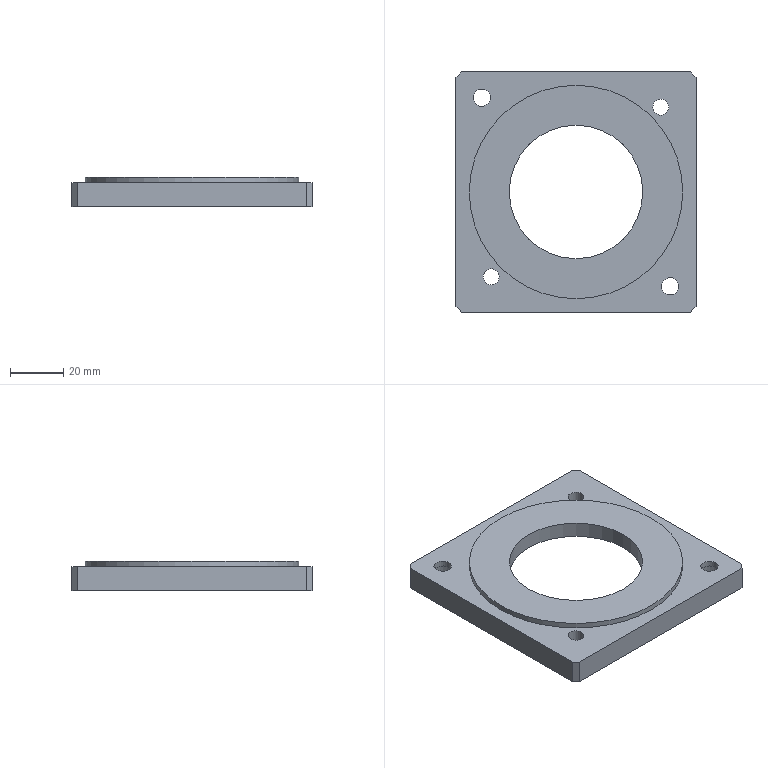Part | NX | 1 solid | 23 faces | box 90 x 90 x 11 mm | volume 49910 mm3 | plane 14 | cylinder 9 | commonest cylinder face diameters 6 x2 6.5 x2 11 x2 50 x1 70 x1 80 x1
STEP:
#1=CARTESIAN_POINT('',(-34.82,-31.82,-11.));
#2=VERTEX_POINT('',#1);
#3=CARTESIAN_POINT('',(-31.82,-31.82,-11.));
#4=DIRECTION('',(0.,0.,1.));
#5=DIRECTION('',(-1.,0.,0.));
#6=AXIS2_PLACEMENT_3D('',#3,#4,#5);
#7=CIRCLE('',#6,3.);
#8=EDGE_CURVE('',#2,#2,#7,.T.);
#9=ORIENTED_EDGE('',*,*,#8,.F.);
#10=EDGE_LOOP('',(#9));
#11=FACE_BOUND('',#10,.T.);
#12=CARTESIAN_POINT('',(-28.82,-31.82,-2.));
#13=VERTEX_POINT('',#12);
#14=CARTESIAN_POINT('',(-31.82,-31.82,-2.));
#15=DIRECTION('',(0.,0.,1.));
#16=DIRECTION('',(1.,0.,0.));
#17=AXIS2_PLACEMENT_3D('',#14,#15,#16);
#18=CIRCLE('',#17,3.);
#19=EDGE_CURVE('',#13,#13,#18,.F.);
#20=ORIENTED_EDGE('',*,*,#19,.F.);
#21=EDGE_LOOP('',(#20));
#22=FACE_BOUND('',#21,.T.);
#23=CARTESIAN_POINT('',(-31.82,-31.82,-11.));
#24=DIRECTION('',(0.,0.,1.));
#25=DIRECTION('',(1.,0.,0.));
#26=AXIS2_PLACEMENT_3D('',#23,#24,#25);
#27=CYLINDRICAL_SURFACE('',#26,3.);
#28=ADVANCED_FACE('',(#11,#22),#27,.F.);
#29=CARTESIAN_POINT('',(34.82,31.82,-11.));
#30=VERTEX_POINT('',#29);
#31=CARTESIAN_POINT('',(31.82,31.82,-11.));
#32=DIRECTION('',(0.,0.,1.));
#33=DIRECTION('',(1.,0.,0.));
#34=AXIS2_PLACEMENT_3D('',#31,#32,#33);
#35=CIRCLE('',#34,3.);
#36=EDGE_CURVE('',#30,#30,#35,.T.);
#37=ORIENTED_EDGE('',*,*,#36,.F.);
#38=EDGE_LOOP('',(#37));
#39=FACE_BOUND('',#38,.T.);
#40=CARTESIAN_POINT('',(34.82,31.82,-2.));
#41=VERTEX_POINT('',#40);
#42=CARTESIAN_POINT('',(31.82,31.82,-2.));
#43=DIRECTION('',(0.,0.,1.));
#44=DIRECTION('',(1.,0.,0.));
#45=AXIS2_PLACEMENT_3D('',#42,#43,#44);
#46=CIRCLE('',#45,3.);
#47=EDGE_CURVE('',#41,#41,#46,.F.);
#48=ORIENTED_EDGE('',*,*,#47,.F.);
#49=EDGE_LOOP('',(#48));
#50=FACE_BOUND('',#49,.T.);
#51=CARTESIAN_POINT('',(31.82,31.82,-11.));
#52=DIRECTION('',(0.,0.,1.));
#53=DIRECTION('',(1.,0.,0.));
#54=AXIS2_PLACEMENT_3D('',#51,#52,#53);
#55=CYLINDRICAL_SURFACE('',#54,3.);
#56=ADVANCED_FACE('',(#39,#50),#55,.F.);
#57=CARTESIAN_POINT('',(38.605,-35.355,-4.2));
#58=VERTEX_POINT('',#57);
#59=CARTESIAN_POINT('',(35.355,-35.355,-4.2));
#60=DIRECTION('',(0.,0.,1.));
#61=DIRECTION('',(1.,0.,0.));
#62=AXIS2_PLACEMENT_3D('',#59,#60,#61);
#63=CIRCLE('',#62,3.25);
#64=EDGE_CURVE('',#58,#58,#63,.F.);
#65=ORIENTED_EDGE('',*,*,#64,.T.);
#66=EDGE_LOOP('',(#65));
#67=FACE_BOUND('',#66,.T.);
#68=CARTESIAN_POINT('',(38.605,-35.355,-2.));
#69=VERTEX_POINT('',#68);
#70=CARTESIAN_POINT('',(35.355,-35.355,-2.));
#71=DIRECTION('',(0.,0.,1.));
#72=DIRECTION('',(1.,0.,0.));
#73=AXIS2_PLACEMENT_3D('',#70,#71,#72);
#74=CIRCLE('',#73,3.25);
#75=EDGE_CURVE('',#69,#69,#74,.F.);
#76=ORIENTED_EDGE('',*,*,#75,.F.);
#77=EDGE_LOOP('',(#76));
#78=FACE_BOUND('',#77,.T.);
#79=CARTESIAN_POINT('',(35.355,-35.355,-11.));
#80=DIRECTION('',(0.,0.,1.));
#81=DIRECTION('',(1.,0.,0.));
#82=AXIS2_PLACEMENT_3D('',#79,#80,#81);
#83=CYLINDRICAL_SURFACE('',#82,3.25);
#84=ADVANCED_FACE('',(#67,#78),#83,.F.);
#85=CARTESIAN_POINT('',(-32.105,35.355,-4.2));
#86=VERTEX_POINT('',#85);
#87=CARTESIAN_POINT('',(-35.355,35.355,-4.2));
#88=DIRECTION('',(0.,0.,1.));
#89=DIRECTION('',(1.,0.,0.));
#90=AXIS2_PLACEMENT_3D('',#87,#88,#89);
#91=CIRCLE('',#90,3.25);
#92=EDGE_CURVE('',#86,#86,#91,.F.);
#93=ORIENTED_EDGE('',*,*,#92,.T.);
#94=EDGE_LOOP('',(#93));
#95=FACE_BOUND('',#94,.T.);
#96=CARTESIAN_POINT('',(-32.105,35.355,-2.));
#97=VERTEX_POINT('',#96);
#98=CARTESIAN_POINT('',(-35.355,35.355,-2.));
#99=DIRECTION('',(0.,0.,1.));
#100=DIRECTION('',(1.,0.,0.));
#101=AXIS2_PLACEMENT_3D('',#98,#99,#100);
#102=CIRCLE('',#101,3.25);
#103=EDGE_CURVE('',#97,#97,#102,.F.);
#104=ORIENTED_EDGE('',*,*,#103,.F.);
#105=EDGE_LOOP('',(#104));
#106=FACE_BOUND('',#105,.T.);
#107=CARTESIAN_POINT('',(-35.355,35.355,-11.));
#108=DIRECTION('',(0.,0.,1.));
#109=DIRECTION('',(1.,0.,0.));
#110=AXIS2_PLACEMENT_3D('',#107,#108,#109);
#111=CYLINDRICAL_SURFACE('',#110,3.25);
#112=ADVANCED_FACE('',(#95,#106),#111,.F.);
#113=CARTESIAN_POINT('',(25.,0.,0.));
#114=VERTEX_POINT('',#113);
#115=CARTESIAN_POINT('',(0.,0.,0.));
#116=DIRECTION('',(0.,0.,1.));
#117=DIRECTION('',(1.,0.,0.));
#118=AXIS2_PLACEMENT_3D('',#115,#116,#117);
#119=CIRCLE('',#118,25.);
#120=EDGE_CURVE('',#114,#114,#119,.T.);
#121=ORIENTED_EDGE('',*,*,#120,.F.);
#122=EDGE_LOOP('',(#121));
#123=FACE_BOUND('',#122,.T.);
#124=CARTESIAN_POINT('',(40.,0.,0.));
#125=VERTEX_POINT('',#124);
#126=CARTESIAN_POINT('',(0.,0.,0.));
#127=DIRECTION('',(0.,0.,1.));
#128=DIRECTION('',(1.,0.,0.));
#129=AXIS2_PLACEMENT_3D('',#126,#127,#128);
#130=CIRCLE('',#129,40.);
#131=EDGE_CURVE('',#125,#125,#130,.T.);
#132=ORIENTED_EDGE('',*,*,#131,.T.);
#133=EDGE_LOOP('',(#132));
#134=FACE_BOUND('',#133,.T.);
#135=CARTESIAN_POINT('',(35.355,-35.355,0.));
#136=DIRECTION('',(0.,0.,1.));
#137=DIRECTION('',(1.,0.,0.));
#138=AXIS2_PLACEMENT_3D('',#135,#136,#137);
#139=PLANE('',#138);
#140=ADVANCED_FACE('',(#123,#134),#139,.T.);
#141=CARTESIAN_POINT('',(-43.,45.,-2.));
#142=VERTEX_POINT('',#141);
#143=CARTESIAN_POINT('',(-45.,43.,-2.));
#144=VERTEX_POINT('',#143);
#145=CARTESIAN_POINT('',(-43.,45.,-2.));
#146=CARTESIAN_POINT('',(-45.,43.,-2.));
#147=B_SPLINE_CURVE_WITH_KNOTS('',1,(#145,#146),.UNSPECIFIED.,.F.,.F.,(2,2),(0.,0.125),.PIECEWISE_BEZIER_KNOTS.);
#148=EDGE_CURVE('',#142,#144,#147,.T.);
#149=ORIENTED_EDGE('',*,*,#148,.F.);
#150=CARTESIAN_POINT('',(-43.,45.,-11.));
#151=VERTEX_POINT('',#150);
#152=CARTESIAN_POINT('',(-43.,45.,-11.));
#153=DIRECTION('',(0.,0.,1.));
#154=VECTOR('',#153,1000.);
#155=LINE('',#152,#154);
#156=EDGE_CURVE('',#151,#142,#155,.T.);
#157=ORIENTED_EDGE('',*,*,#156,.F.);
#158=CARTESIAN_POINT('',(-45.,43.,-11.));
#159=VERTEX_POINT('',#158);
#160=CARTESIAN_POINT('',(-43.,45.,-11.));
#161=CARTESIAN_POINT('',(-45.,43.,-11.));
#162=B_SPLINE_CURVE_WITH_KNOTS('',1,(#160,#161),.UNSPECIFIED.,.F.,.F.,(2,2),(0.,0.125),.PIECEWISE_BEZIER_KNOTS.);
#163=EDGE_CURVE('',#151,#159,#162,.T.);
#164=ORIENTED_EDGE('',*,*,#163,.T.);
#165=CARTESIAN_POINT('',(-45.,43.,-11.));
#166=DIRECTION('',(0.,0.,1.));
#167=VECTOR('',#166,1000.);
#168=LINE('',#165,#167);
#169=EDGE_CURVE('',#159,#144,#168,.T.);
#170=ORIENTED_EDGE('',*,*,#169,.T.);
#171=EDGE_LOOP('',(#149,#157,#164,#170));
#172=FACE_BOUND('',#171,.T.);
#173=CARTESIAN_POINT('',(-43.,45.,-11.));
#174=DIRECTION('',(-0.7071,0.7071,0.));
#175=DIRECTION('',(-0.7071,-0.7071,0.));
#176=AXIS2_PLACEMENT_3D('',#173,#174,#175);
#177=PLANE('',#176);
#178=ADVANCED_FACE('',(#172),#177,.T.);
#179=CARTESIAN_POINT('',(-45.,-43.,-2.));
#180=VERTEX_POINT('',#179);
#181=CARTESIAN_POINT('',(-45.,43.,-2.));
#182=CARTESIAN_POINT('',(-45.,-43.,-2.));
#183=B_SPLINE_CURVE_WITH_KNOTS('',1,(#181,#182),.UNSPECIFIED.,.F.,.F.,(2,2),(0.125,0.25),.PIECEWISE_BEZIER_KNOTS.);
#184=EDGE_CURVE('',#144,#180,#183,.T.);
#185=ORIENTED_EDGE('',*,*,#184,.F.);
#186=ORIENTED_EDGE('',*,*,#169,.F.);
#187=CARTESIAN_POINT('',(-45.,-43.,-11.));
#188=VERTEX_POINT('',#187);
#189=CARTESIAN_POINT('',(-45.,43.,-11.));
#190=CARTESIAN_POINT('',(-45.,-43.,-11.));
#191=B_SPLINE_CURVE_WITH_KNOTS('',1,(#189,#190),.UNSPECIFIED.,.F.,.F.,(2,2),(0.125,0.25),.PIECEWISE_BEZIER_KNOTS.);
#192=EDGE_CURVE('',#159,#188,#191,.T.);
#193=ORIENTED_EDGE('',*,*,#192,.T.);
#194=CARTESIAN_POINT('',(-45.,-43.,-11.));
#195=DIRECTION('',(0.,0.,1.));
#196=VECTOR('',#195,1000.);
#197=LINE('',#194,#196);
#198=EDGE_CURVE('',#188,#180,#197,.T.);
#199=ORIENTED_EDGE('',*,*,#198,.T.);
#200=EDGE_LOOP('',(#185,#186,#193,#199));
#201=FACE_BOUND('',#200,.T.);
#202=CARTESIAN_POINT('',(-45.,43.,-11.));
#203=DIRECTION('',(-1.,0.,0.));
#204=DIRECTION('',(0.,-1.,0.));
#205=AXIS2_PLACEMENT_3D('',#202,#203,#204);
#206=PLANE('',#205);
#207=ADVANCED_FACE('',(#201),#206,.T.);
#208=CARTESIAN_POINT('',(-43.,-45.,-2.));
#209=VERTEX_POINT('',#208);
#210=CARTESIAN_POINT('',(-45.,-43.,-2.));
#211=CARTESIAN_POINT('',(-43.,-45.,-2.));
#212=B_SPLINE_CURVE_WITH_KNOTS('',1,(#210,#211),.UNSPECIFIED.,.F.,.F.,(2,2),(0.25,0.375),.PIECEWISE_BEZIER_KNOTS.);
#213=EDGE_CURVE('',#180,#209,#212,.T.);
#214=ORIENTED_EDGE('',*,*,#213,.F.);
#215=ORIENTED_EDGE('',*,*,#198,.F.);
#216=CARTESIAN_POINT('',(-43.,-45.,-11.));
#217=VERTEX_POINT('',#216);
#218=CARTESIAN_POINT('',(-45.,-43.,-11.));
#219=CARTESIAN_POINT('',(-43.,-45.,-11.));
#220=B_SPLINE_CURVE_WITH_KNOTS('',1,(#218,#219),.UNSPECIFIED.,.F.,.F.,(2,2),(0.25,0.375),.PIECEWISE_BEZIER_KNOTS.);
#221=EDGE_CURVE('',#188,#217,#220,.T.);
#222=ORIENTED_EDGE('',*,*,#221,.T.);
#223=CARTESIAN_POINT('',(-43.,-45.,-11.));
#224=DIRECTION('',(0.,0.,1.));
#225=VECTOR('',#224,1000.);
#226=LINE('',#223,#225);
#227=EDGE_CURVE('',#217,#209,#226,.T.);
#228=ORIENTED_EDGE('',*,*,#227,.T.);
#229=EDGE_LOOP('',(#214,#215,#222,#228));
#230=FACE_BOUND('',#229,.T.);
#231=CARTESIAN_POINT('',(-45.,-43.,-11.));
#232=DIRECTION('',(-0.7071,-0.7071,0.));
#233=DIRECTION('',(0.7071,-0.7071,0.));
#234=AXIS2_PLACEMENT_3D('',#231,#232,#233);
#235=PLANE('',#234);
#236=ADVANCED_FACE('',(#230),#235,.T.);
#237=CARTESIAN_POINT('',(43.,-45.,-2.));
#238=VERTEX_POINT('',#237);
#239=CARTESIAN_POINT('',(-43.,-45.,-2.));
#240=CARTESIAN_POINT('',(43.,-45.,-2.));
#241=B_SPLINE_CURVE_WITH_KNOTS('',1,(#239,#240),.UNSPECIFIED.,.F.,.F.,(2,2),(0.375,0.5),.PIECEWISE_BEZIER_KNOTS.);
#242=EDGE_CURVE('',#209,#238,#241,.T.);
#243=ORIENTED_EDGE('',*,*,#242,.F.);
#244=ORIENTED_EDGE('',*,*,#227,.F.);
#245=CARTESIAN_POINT('',(43.,-45.,-11.));
#246=VERTEX_POINT('',#245);
#247=CARTESIAN_POINT('',(-43.,-45.,-11.));
#248=CARTESIAN_POINT('',(43.,-45.,-11.));
#249=B_SPLINE_CURVE_WITH_KNOTS('',1,(#247,#248),.UNSPECIFIED.,.F.,.F.,(2,2),(0.375,0.5),.PIECEWISE_BEZIER_KNOTS.);
#250=EDGE_CURVE('',#217,#246,#249,.T.);
#251=ORIENTED_EDGE('',*,*,#250,.T.);
#252=CARTESIAN_POINT('',(43.,-45.,-11.));
#253=DIRECTION('',(0.,0.,1.));
#254=VECTOR('',#253,1000.);
#255=LINE('',#252,#254);
#256=EDGE_CURVE('',#246,#238,#255,.T.);
#257=ORIENTED_EDGE('',*,*,#256,.T.);
#258=EDGE_LOOP('',(#243,#244,#251,#257));
#259=FACE_BOUND('',#258,.T.);
#260=CARTESIAN_POINT('',(-43.,-45.,-11.));
#261=DIRECTION('',(0.,-1.,0.));
#262=DIRECTION('',(1.,0.,0.));
#263=AXIS2_PLACEMENT_3D('',#260,#261,#262);
#264=PLANE('',#263);
#265=ADVANCED_FACE('',(#259),#264,.T.);
#266=CARTESIAN_POINT('',(45.,-43.,-2.));
#267=VERTEX_POINT('',#266);
#268=CARTESIAN_POINT('',(43.,-45.,-2.));
#269=CARTESIAN_POINT('',(45.,-43.,-2.));
#270=B_SPLINE_CURVE_WITH_KNOTS('',1,(#268,#269),.UNSPECIFIED.,.F.,.F.,(2,2),(0.5,0.625),.PIECEWISE_BEZIER_KNOTS.);
#271=EDGE_CURVE('',#238,#267,#270,.T.);
#272=ORIENTED_EDGE('',*,*,#271,.F.);
#273=ORIENTED_EDGE('',*,*,#256,.F.);
#274=CARTESIAN_POINT('',(45.,-43.,-11.));
#275=VERTEX_POINT('',#274);
#276=CARTESIAN_POINT('',(43.,-45.,-11.));
#277=CARTESIAN_POINT('',(45.,-43.,-11.));
#278=B_SPLINE_CURVE_WITH_KNOTS('',1,(#276,#277),.UNSPECIFIED.,.F.,.F.,(2,2),(0.5,0.625),.PIECEWISE_BEZIER_KNOTS.);
#279=EDGE_CURVE('',#246,#275,#278,.T.);
#280=ORIENTED_EDGE('',*,*,#279,.T.);
#281=CARTESIAN_POINT('',(45.,-43.,-11.));
#282=DIRECTION('',(0.,0.,1.));
#283=VECTOR('',#282,1000.);
#284=LINE('',#281,#283);
#285=EDGE_CURVE('',#275,#267,#284,.T.);
#286=ORIENTED_EDGE('',*,*,#285,.T.);
#287=EDGE_LOOP('',(#272,#273,#280,#286));
#288=FACE_BOUND('',#287,.T.);
#289=CARTESIAN_POINT('',(43.,-45.,-11.));
#290=DIRECTION('',(0.7071,-0.7071,0.));
#291=DIRECTION('',(0.7071,0.7071,0.));
#292=AXIS2_PLACEMENT_3D('',#289,#290,#291);
#293=PLANE('',#292);
#294=ADVANCED_FACE('',(#288),#293,.T.);
#295=CARTESIAN_POINT('',(45.,43.,-2.));
#296=VERTEX_POINT('',#295);
#297=CARTESIAN_POINT('',(45.,-43.,-2.));
#298=CARTESIAN_POINT('',(45.,43.,-2.));
#299=B_SPLINE_CURVE_WITH_KNOTS('',1,(#297,#298),.UNSPECIFIED.,.F.,.F.,(2,2),(0.625,0.75),.PIECEWISE_BEZIER_KNOTS.);
#300=EDGE_CURVE('',#267,#296,#299,.T.);
#301=ORIENTED_EDGE('',*,*,#300,.F.);
#302=ORIENTED_EDGE('',*,*,#285,.F.);
#303=CARTESIAN_POINT('',(45.,43.,-11.));
#304=VERTEX_POINT('',#303);
#305=CARTESIAN_POINT('',(45.,-43.,-11.));
#306=CARTESIAN_POINT('',(45.,43.,-11.));
#307=B_SPLINE_CURVE_WITH_KNOTS('',1,(#305,#306),.UNSPECIFIED.,.F.,.F.,(2,2),(0.625,0.75),.PIECEWISE_BEZIER_KNOTS.);
#308=EDGE_CURVE('',#275,#304,#307,.T.);
#309=ORIENTED_EDGE('',*,*,#308,.T.);
#310=CARTESIAN_POINT('',(45.,43.,-11.));
#311=DIRECTION('',(0.,0.,1.));
#312=VECTOR('',#311,1000.);
#313=LINE('',#310,#312);
#314=EDGE_CURVE('',#304,#296,#313,.T.);
#315=ORIENTED_EDGE('',*,*,#314,.T.);
#316=EDGE_LOOP('',(#301,#302,#309,#315));
#317=FACE_BOUND('',#316,.T.);
#318=CARTESIAN_POINT('',(45.,-43.,-11.));
#319=DIRECTION('',(1.,0.,0.));
#320=DIRECTION('',(0.,0.,-1.));
#321=AXIS2_PLACEMENT_3D('',#318,#319,#320);
#322=PLANE('',#321);
#323=ADVANCED_FACE('',(#317),#322,.T.);
#324=CARTESIAN_POINT('',(43.,45.,-2.));
#325=VERTEX_POINT('',#324);
#326=CARTESIAN_POINT('',(45.,43.,-2.));
#327=CARTESIAN_POINT('',(43.,45.,-2.));
#328=B_SPLINE_CURVE_WITH_KNOTS('',1,(#326,#327),.UNSPECIFIED.,.F.,.F.,(2,2),(0.75,0.875),.PIECEWISE_BEZIER_KNOTS.);
#329=EDGE_CURVE('',#296,#325,#328,.T.);
#330=ORIENTED_EDGE('',*,*,#329,.F.);
#331=ORIENTED_EDGE('',*,*,#314,.F.);
#332=CARTESIAN_POINT('',(43.,45.,-11.));
#333=VERTEX_POINT('',#332);
#334=CARTESIAN_POINT('',(45.,43.,-11.));
#335=CARTESIAN_POINT('',(43.,45.,-11.));
#336=B_SPLINE_CURVE_WITH_KNOTS('',1,(#334,#335),.UNSPECIFIED.,.F.,.F.,(2,2),(0.75,0.875),.PIECEWISE_BEZIER_KNOTS.);
#337=EDGE_CURVE('',#304,#333,#336,.T.);
#338=ORIENTED_EDGE('',*,*,#337,.T.);
#339=CARTESIAN_POINT('',(43.,45.,-11.));
#340=DIRECTION('',(0.,0.,1.));
#341=VECTOR('',#340,1000.);
#342=LINE('',#339,#341);
#343=EDGE_CURVE('',#333,#325,#342,.T.);
#344=ORIENTED_EDGE('',*,*,#343,.T.);
#345=EDGE_LOOP('',(#330,#331,#338,#344));
#346=FACE_BOUND('',#345,.T.);
#347=CARTESIAN_POINT('',(45.,43.,-11.));
#348=DIRECTION('',(0.7071,0.7071,0.));
#349=DIRECTION('',(-0.7071,0.7071,0.));
#350=AXIS2_PLACEMENT_3D('',#347,#348,#349);
#351=PLANE('',#350);
#352=ADVANCED_FACE('',(#346),#351,.T.);
#353=CARTESIAN_POINT('',(25.,0.,-6.));
#354=VERTEX_POINT('',#353);
#355=CARTESIAN_POINT('',(0.,0.,-6.));
#356=DIRECTION('',(0.,0.,1.));
#357=DIRECTION('',(1.,0.,0.));
#358=AXIS2_PLACEMENT_3D('',#355,#356,#357);
#359=CIRCLE('',#358,25.);
#360=EDGE_CURVE('',#354,#354,#359,.F.);
#361=ORIENTED_EDGE('',*,*,#360,.T.);
#362=EDGE_LOOP('',(#361));
#363=FACE_BOUND('',#362,.T.);
#364=ORIENTED_EDGE('',*,*,#120,.T.);
#365=EDGE_LOOP('',(#364));
#366=FACE_BOUND('',#365,.T.);
#367=CARTESIAN_POINT('',(0.,0.,-11.));
#368=DIRECTION('',(0.,0.,1.));
#369=DIRECTION('',(1.,0.,0.));
#370=AXIS2_PLACEMENT_3D('',#367,#368,#369);
#371=CYLINDRICAL_SURFACE('',#370,25.);
#372=ADVANCED_FACE('',(#363,#366),#371,.F.);
#373=CARTESIAN_POINT('',(43.,45.,-2.));
#374=CARTESIAN_POINT('',(-43.,45.,-2.));
#375=B_SPLINE_CURVE_WITH_KNOTS('',1,(#373,#374),.UNSPECIFIED.,.F.,.F.,(2,2),(0.875,1.),.PIECEWISE_BEZIER_KNOTS.);
#376=EDGE_CURVE('',#325,#142,#375,.T.);
#377=ORIENTED_EDGE('',*,*,#376,.F.);
#378=ORIENTED_EDGE('',*,*,#343,.F.);
#379=CARTESIAN_POINT('',(43.,45.,-11.));
#380=CARTESIAN_POINT('',(-43.,45.,-11.));
#381=B_SPLINE_CURVE_WITH_KNOTS('',1,(#379,#380),.UNSPECIFIED.,.F.,.F.,(2,2),(0.875,1.),.PIECEWISE_BEZIER_KNOTS.);
#382=EDGE_CURVE('',#333,#151,#381,.T.);
#383=ORIENTED_EDGE('',*,*,#382,.T.);
#384=ORIENTED_EDGE('',*,*,#156,.T.);
#385=EDGE_LOOP('',(#377,#378,#383,#384));
#386=FACE_BOUND('',#385,.T.);
#387=CARTESIAN_POINT('',(43.,45.,-11.));
#388=DIRECTION('',(0.,1.,0.));
#389=DIRECTION('',(0.,0.,1.));
#390=AXIS2_PLACEMENT_3D('',#387,#388,#389);
#391=PLANE('',#390);
#392=ADVANCED_FACE('',(#386),#391,.T.);
#393=CARTESIAN_POINT('',(35.,0.,-11.));
#394=VERTEX_POINT('',#393);
#395=CARTESIAN_POINT('',(0.,0.,-11.));
#396=DIRECTION('',(0.,0.,1.));
#397=DIRECTION('',(1.,0.,0.));
#398=AXIS2_PLACEMENT_3D('',#395,#396,#397);
#399=CIRCLE('',#398,35.);
#400=EDGE_CURVE('',#394,#394,#399,.T.);
#401=ORIENTED_EDGE('',*,*,#400,.T.);
#402=EDGE_LOOP('',(#401));
#403=FACE_BOUND('',#402,.T.);
#404=CARTESIAN_POINT('',(40.855,-35.355,-11.));
#405=VERTEX_POINT('',#404);
#406=CARTESIAN_POINT('',(35.355,-35.355,-11.));
#407=DIRECTION('',(0.,0.,1.));
#408=DIRECTION('',(1.,0.,0.));
#409=AXIS2_PLACEMENT_3D('',#406,#407,#408);
#410=CIRCLE('',#409,5.5);
#411=EDGE_CURVE('',#405,#405,#410,.T.);
#412=ORIENTED_EDGE('',*,*,#411,.T.);
#413=EDGE_LOOP('',(#412));
#414=FACE_BOUND('',#413,.T.);
#415=CARTESIAN_POINT('',(-29.855,35.355,-11.));
#416=VERTEX_POINT('',#415);
#417=CARTESIAN_POINT('',(-35.355,35.355,-11.));
#418=DIRECTION('',(0.,0.,1.));
#419=DIRECTION('',(1.,0.,0.));
#420=AXIS2_PLACEMENT_3D('',#417,#418,#419);
#421=CIRCLE('',#420,5.5);
#422=EDGE_CURVE('',#416,#416,#421,.T.);
#423=ORIENTED_EDGE('',*,*,#422,.T.);
#424=EDGE_LOOP('',(#423));
#425=FACE_BOUND('',#424,.T.);
#426=ORIENTED_EDGE('',*,*,#163,.F.);
#427=ORIENTED_EDGE('',*,*,#382,.F.);
#428=ORIENTED_EDGE('',*,*,#337,.F.);
#429=ORIENTED_EDGE('',*,*,#308,.F.);
#430=ORIENTED_EDGE('',*,*,#279,.F.);
#431=ORIENTED_EDGE('',*,*,#250,.F.);
#432=ORIENTED_EDGE('',*,*,#221,.F.);
#433=ORIENTED_EDGE('',*,*,#192,.F.);
#434=EDGE_LOOP('',(#426,#427,#428,#429,#430,#431,#432,#433));
#435=FACE_BOUND('',#434,.T.);
#436=ORIENTED_EDGE('',*,*,#36,.T.);
#437=EDGE_LOOP('',(#436));
#438=FACE_BOUND('',#437,.T.);
#439=ORIENTED_EDGE('',*,*,#8,.T.);
#440=EDGE_LOOP('',(#439));
#441=FACE_BOUND('',#440,.T.);
#442=CARTESIAN_POINT('',(35.355,-35.355,-11.));
#443=DIRECTION('',(0.,0.,1.));
#444=DIRECTION('',(1.,0.,0.));
#445=AXIS2_PLACEMENT_3D('',#442,#443,#444);
#446=PLANE('',#445);
#447=ADVANCED_FACE('',(#403,#414,#425,#435,#438,#441),#446,.F.);
#448=ORIENTED_EDGE('',*,*,#148,.T.);
#449=ORIENTED_EDGE('',*,*,#184,.T.);
#450=ORIENTED_EDGE('',*,*,#213,.T.);
#451=ORIENTED_EDGE('',*,*,#242,.T.);
#452=ORIENTED_EDGE('',*,*,#271,.T.);
#453=ORIENTED_EDGE('',*,*,#300,.T.);
#454=ORIENTED_EDGE('',*,*,#329,.T.);
#455=ORIENTED_EDGE('',*,*,#376,.T.);
#456=EDGE_LOOP('',(#448,#449,#450,#451,#452,#453,#454,#455));
#457=FACE_BOUND('',#456,.T.);
#458=CARTESIAN_POINT('',(40.,0.,-2.));
#459=VERTEX_POINT('',#458);
#460=CARTESIAN_POINT('',(0.,0.,-2.));
#461=DIRECTION('',(0.,0.,1.));
#462=DIRECTION('',(1.,0.,0.));
#463=AXIS2_PLACEMENT_3D('',#460,#461,#462);
#464=CIRCLE('',#463,40.);
#465=EDGE_CURVE('',#459,#459,#464,.F.);
#466=ORIENTED_EDGE('',*,*,#465,.T.);
#467=EDGE_LOOP('',(#466));
#468=FACE_BOUND('',#467,.T.);
#469=ORIENTED_EDGE('',*,*,#103,.T.);
#470=EDGE_LOOP('',(#469));
#471=FACE_BOUND('',#470,.T.);
#472=ORIENTED_EDGE('',*,*,#75,.T.);
#473=EDGE_LOOP('',(#472));
#474=FACE_BOUND('',#473,.T.);
#475=ORIENTED_EDGE('',*,*,#47,.T.);
#476=EDGE_LOOP('',(#475));
#477=FACE_BOUND('',#476,.T.);
#478=ORIENTED_EDGE('',*,*,#19,.T.);
#479=EDGE_LOOP('',(#478));
#480=FACE_BOUND('',#479,.T.);
#481=CARTESIAN_POINT('',(0.,0.,-2.));
#482=DIRECTION('',(0.,0.,1.));
#483=DIRECTION('',(1.,0.,0.));
#484=AXIS2_PLACEMENT_3D('',#481,#482,#483);
#485=PLANE('',#484);
#486=ADVANCED_FACE('',(#457,#468,#471,#474,#477,#480),#485,.T.);
#487=ORIENTED_EDGE('',*,*,#465,.F.);
#488=EDGE_LOOP('',(#487));
#489=FACE_BOUND('',#488,.T.);
#490=ORIENTED_EDGE('',*,*,#131,.F.);
#491=EDGE_LOOP('',(#490));
#492=FACE_BOUND('',#491,.T.);
#493=CARTESIAN_POINT('',(0.,0.,-2.));
#494=DIRECTION('',(0.,0.,1.));
#495=DIRECTION('',(1.,0.,0.));
#496=AXIS2_PLACEMENT_3D('',#493,#494,#495);
#497=CYLINDRICAL_SURFACE('',#496,40.);
#498=ADVANCED_FACE('',(#489,#492),#497,.T.);
#499=CARTESIAN_POINT('',(-29.855,35.355,-4.2));
#500=VERTEX_POINT('',#499);
#501=CARTESIAN_POINT('',(-35.355,35.355,-4.2));
#502=DIRECTION('',(0.,0.,1.));
#503=DIRECTION('',(1.,0.,0.));
#504=AXIS2_PLACEMENT_3D('',#501,#502,#503);
#505=CIRCLE('',#504,5.5);
#506=EDGE_CURVE('',#500,#500,#505,.F.);
#507=ORIENTED_EDGE('',*,*,#506,.T.);
#508=EDGE_LOOP('',(#507));
#509=FACE_BOUND('',#508,.T.);
#510=ORIENTED_EDGE('',*,*,#92,.F.);
#511=EDGE_LOOP('',(#510));
#512=FACE_BOUND('',#511,.T.);
#513=CARTESIAN_POINT('',(-35.355,35.355,-4.2));
#514=DIRECTION('',(0.,0.,1.));
#515=DIRECTION('',(1.,0.,0.));
#516=AXIS2_PLACEMENT_3D('',#513,#514,#515);
#517=PLANE('',#516);
#518=ADVANCED_FACE('',(#509,#512),#517,.F.);
#519=ORIENTED_EDGE('',*,*,#422,.F.);
#520=EDGE_LOOP('',(#519));
#521=FACE_BOUND('',#520,.T.);
#522=ORIENTED_EDGE('',*,*,#506,.F.);
#523=EDGE_LOOP('',(#522));
#524=FACE_BOUND('',#523,.T.);
#525=CARTESIAN_POINT('',(-35.355,35.355,-11.));
#526=DIRECTION('',(0.,0.,1.));
#527=DIRECTION('',(1.,0.,0.));
#528=AXIS2_PLACEMENT_3D('',#525,#526,#527);
#529=CYLINDRICAL_SURFACE('',#528,5.5);
#530=ADVANCED_FACE('',(#521,#524),#529,.F.);
#531=CARTESIAN_POINT('',(40.855,-35.355,-4.2));
#532=VERTEX_POINT('',#531);
#533=CARTESIAN_POINT('',(35.355,-35.355,-4.2));
#534=DIRECTION('',(0.,0.,1.));
#535=DIRECTION('',(1.,0.,0.));
#536=AXIS2_PLACEMENT_3D('',#533,#534,#535);
#537=CIRCLE('',#536,5.5);
#538=EDGE_CURVE('',#532,#532,#537,.F.);
#539=ORIENTED_EDGE('',*,*,#538,.T.);
#540=EDGE_LOOP('',(#539));
#541=FACE_BOUND('',#540,.T.);
#542=ORIENTED_EDGE('',*,*,#64,.F.);
#543=EDGE_LOOP('',(#542));
#544=FACE_BOUND('',#543,.T.);
#545=CARTESIAN_POINT('',(35.355,-35.355,-4.2));
#546=DIRECTION('',(0.,0.,1.));
#547=DIRECTION('',(1.,0.,0.));
#548=AXIS2_PLACEMENT_3D('',#545,#546,#547);
#549=PLANE('',#548);
#550=ADVANCED_FACE('',(#541,#544),#549,.F.);
#551=ORIENTED_EDGE('',*,*,#411,.F.);
#552=EDGE_LOOP('',(#551));
#553=FACE_BOUND('',#552,.T.);
#554=ORIENTED_EDGE('',*,*,#538,.F.);
#555=EDGE_LOOP('',(#554));
#556=FACE_BOUND('',#555,.T.);
#557=CARTESIAN_POINT('',(35.355,-35.355,-11.));
#558=DIRECTION('',(0.,0.,1.));
#559=DIRECTION('',(1.,0.,0.));
#560=AXIS2_PLACEMENT_3D('',#557,#558,#559);
#561=CYLINDRICAL_SURFACE('',#560,5.5);
#562=ADVANCED_FACE('',(#553,#556),#561,.F.);
#563=CARTESIAN_POINT('',(35.,0.,-6.));
#564=VERTEX_POINT('',#563);
#565=CARTESIAN_POINT('',(0.,0.,-6.));
#566=DIRECTION('',(0.,0.,1.));
#567=DIRECTION('',(1.,0.,0.));
#568=AXIS2_PLACEMENT_3D('',#565,#566,#567);
#569=CIRCLE('',#568,35.);
#570=EDGE_CURVE('',#564,#564,#569,.F.);
#571=ORIENTED_EDGE('',*,*,#570,.T.);
#572=EDGE_LOOP('',(#571));
#573=FACE_BOUND('',#572,.T.);
#574=ORIENTED_EDGE('',*,*,#360,.F.);
#575=EDGE_LOOP('',(#574));
#576=FACE_BOUND('',#575,.T.);
#577=CARTESIAN_POINT('',(0.,0.,-6.));
#578=DIRECTION('',(0.,0.,1.));
#579=DIRECTION('',(1.,0.,0.));
#580=AXIS2_PLACEMENT_3D('',#577,#578,#579);
#581=PLANE('',#580);
#582=ADVANCED_FACE('',(#573,#576),#581,.F.);
#583=ORIENTED_EDGE('',*,*,#400,.F.);
#584=EDGE_LOOP('',(#583));
#585=FACE_BOUND('',#584,.T.);
#586=ORIENTED_EDGE('',*,*,#570,.F.);
#587=EDGE_LOOP('',(#586));
#588=FACE_BOUND('',#587,.T.);
#589=CARTESIAN_POINT('',(0.,0.,-11.));
#590=DIRECTION('',(0.,0.,1.));
#591=DIRECTION('',(1.,0.,0.));
#592=AXIS2_PLACEMENT_3D('',#589,#590,#591);
#593=CYLINDRICAL_SURFACE('',#592,35.);
#594=ADVANCED_FACE('',(#585,#588),#593,.F.);
#595=CLOSED_SHELL('',(#28,#56,#84,#112,#140,#178,#207,#236,#265,#294,#323,#352,#372,#392,#447,#486,#498,#518,#530,#550,#562,#582,#594));
#596=MANIFOLD_SOLID_BREP('',#595);
#597=(LENGTH_UNIT()NAMED_UNIT(*)SI_UNIT(.MILLI.,.METRE.));
#598=UNCERTAINTY_MEASURE_WITH_UNIT(LENGTH_MEASURE(0.00001),#597,'','');
#599=(NAMED_UNIT(*)PLANE_ANGLE_UNIT()SI_UNIT($,.RADIAN.));
#600=(NAMED_UNIT(*)SI_UNIT($,.STERADIAN.)SOLID_ANGLE_UNIT());
#601=(GEOMETRIC_REPRESENTATION_CONTEXT(3)GLOBAL_UNCERTAINTY_ASSIGNED_CONTEXT((#598))GLOBAL_UNIT_ASSIGNED_CONTEXT((#597,#599,#600))REPRESENTATION_CONTEXT('',''));
#602=ADVANCED_BREP_SHAPE_REPRESENTATION('',(#596),#601);